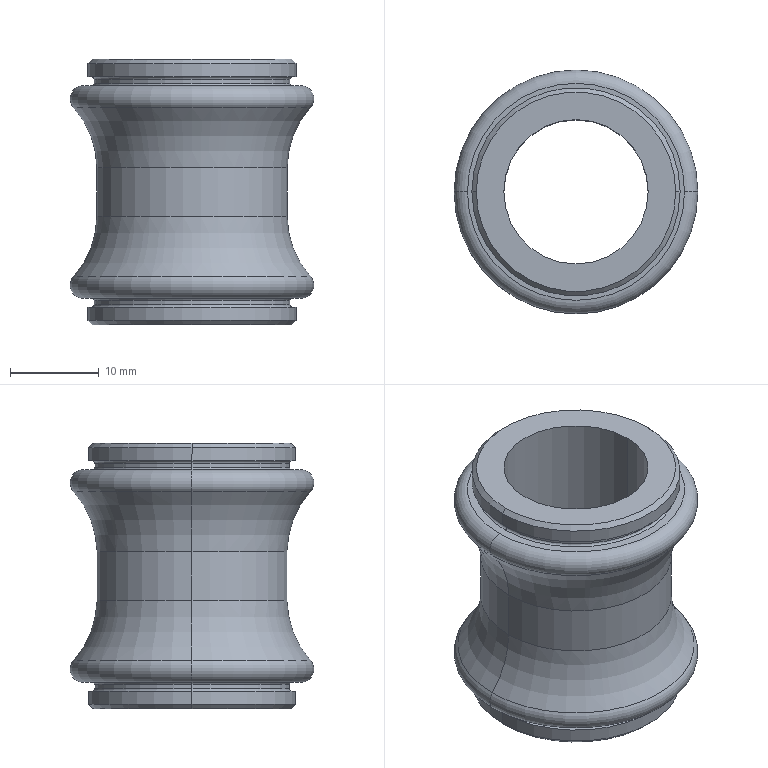Part | SolidWorks | features RefAxis 3, 3DProfileFeature 1, Revolution 1 | 1 solid | 38 faces | box 27.5 x 27.5 x 30 mm | volume 6795 mm3 | torus 16 | cylinder 12 | plane 6 | cone 4 | commonest cylinder face diameters 22.1 x4 23.5 x4 16.3 x2 21.5 x2
STEP:
#1=CARTESIAN_POINT('',(-8.15,0.,0.));
#2=VERTEX_POINT('',#1);
#3=CARTESIAN_POINT('',(8.15,0.,0.));
#4=VERTEX_POINT('',#3);
#5=CARTESIAN_POINT('',(0.,0.,0.));
#6=DIRECTION('',(0.,0.,1.));
#7=DIRECTION('',(1.,0.,0.));
#8=AXIS2_PLACEMENT_3D('',#5,#6,#7);
#9=CIRCLE('',#8,8.15);
#10=EDGE_CURVE('',#2,#4,#9,.T.);
#11=ORIENTED_EDGE('',*,*,#10,.F.);
#12=CARTESIAN_POINT('',(-8.15,0.,30.));
#13=VERTEX_POINT('',#12);
#14=CARTESIAN_POINT('',(-8.15,0.,0.));
#15=DIRECTION('',(0.,0.,1.));
#16=VECTOR('',#15,1000.);
#17=LINE('',#14,#16);
#18=EDGE_CURVE('',#2,#13,#17,.T.);
#19=ORIENTED_EDGE('',*,*,#18,.T.);
#20=CARTESIAN_POINT('',(8.15,0.,30.));
#21=VERTEX_POINT('',#20);
#22=CARTESIAN_POINT('',(0.,0.,30.));
#23=DIRECTION('',(0.,0.,1.));
#24=DIRECTION('',(1.,0.,0.));
#25=AXIS2_PLACEMENT_3D('',#22,#23,#24);
#26=CIRCLE('',#25,8.15);
#27=EDGE_CURVE('',#13,#21,#26,.T.);
#28=ORIENTED_EDGE('',*,*,#27,.T.);
#29=CARTESIAN_POINT('',(8.15,0.,0.));
#30=DIRECTION('',(0.,0.,1.));
#31=VECTOR('',#30,1000.);
#32=LINE('',#29,#31);
#33=EDGE_CURVE('',#4,#21,#32,.T.);
#34=ORIENTED_EDGE('',*,*,#33,.F.);
#35=EDGE_LOOP('',(#11,#19,#28,#34));
#36=FACE_OUTER_BOUND('',#35,.T.);
#37=CARTESIAN_POINT('',(0.,0.,0.));
#38=DIRECTION('',(0.,0.,1.));
#39=DIRECTION('',(1.,0.,0.));
#40=AXIS2_PLACEMENT_3D('',#37,#38,#39);
#41=CYLINDRICAL_SURFACE('',#40,8.15);
#42=ADVANCED_FACE('',(#36),#41,.F.);
#43=CARTESIAN_POINT('',(11.25,0.,0.));
#44=VERTEX_POINT('',#43);
#45=CARTESIAN_POINT('',(-11.25,0.,0.));
#46=VERTEX_POINT('',#45);
#47=CARTESIAN_POINT('',(0.,0.,0.));
#48=DIRECTION('',(0.,0.,1.));
#49=DIRECTION('',(1.,0.,0.));
#50=AXIS2_PLACEMENT_3D('',#47,#48,#49);
#51=CIRCLE('',#50,11.25);
#52=EDGE_CURVE('',#44,#46,#51,.T.);
#53=ORIENTED_EDGE('',*,*,#52,.T.);
#54=CARTESIAN_POINT('',(-11.75,0.,0.5));
#55=VERTEX_POINT('',#54);
#56=CARTESIAN_POINT('',(-11.25,0.,0.));
#57=DIRECTION('',(-0.7071,0.,0.7071));
#58=VECTOR('',#57,1000.);
#59=LINE('',#56,#58);
#60=EDGE_CURVE('',#46,#55,#59,.T.);
#61=ORIENTED_EDGE('',*,*,#60,.T.);
#62=CARTESIAN_POINT('',(11.75,0.,0.5));
#63=VERTEX_POINT('',#62);
#64=CARTESIAN_POINT('',(0.,0.,0.5));
#65=DIRECTION('',(0.,0.,1.));
#66=DIRECTION('',(1.,0.,0.));
#67=AXIS2_PLACEMENT_3D('',#64,#65,#66);
#68=CIRCLE('',#67,11.75);
#69=EDGE_CURVE('',#63,#55,#68,.T.);
#70=ORIENTED_EDGE('',*,*,#69,.F.);
#71=CARTESIAN_POINT('',(11.25,0.,0.));
#72=DIRECTION('',(0.7071,0.,0.7071));
#73=VECTOR('',#72,1000.);
#74=LINE('',#71,#73);
#75=EDGE_CURVE('',#44,#63,#74,.T.);
#76=ORIENTED_EDGE('',*,*,#75,.F.);
#77=EDGE_LOOP('',(#53,#61,#70,#76));
#78=FACE_OUTER_BOUND('',#77,.T.);
#79=CARTESIAN_POINT('',(0.,0.,0.));
#80=DIRECTION('',(0.,0.,1.));
#81=DIRECTION('',(1.,0.,0.));
#82=AXIS2_PLACEMENT_3D('',#79,#80,#81);
#83=CONICAL_SURFACE('',#82,11.25,0.7854);
#84=ADVANCED_FACE('',(#78),#83,.T.);
#85=ORIENTED_EDGE('',*,*,#69,.T.);
#86=CARTESIAN_POINT('',(-11.75,0.,2.));
#87=VERTEX_POINT('',#86);
#88=CARTESIAN_POINT('',(-11.75,0.,0.));
#89=DIRECTION('',(0.,0.,1.));
#90=VECTOR('',#89,1000.);
#91=LINE('',#88,#90);
#92=EDGE_CURVE('',#55,#87,#91,.T.);
#93=ORIENTED_EDGE('',*,*,#92,.T.);
#94=CARTESIAN_POINT('',(11.75,0.,2.));
#95=VERTEX_POINT('',#94);
#96=CARTESIAN_POINT('',(0.,0.,2.));
#97=DIRECTION('',(0.,0.,1.));
#98=DIRECTION('',(1.,0.,0.));
#99=AXIS2_PLACEMENT_3D('',#96,#97,#98);
#100=CIRCLE('',#99,11.75);
#101=EDGE_CURVE('',#95,#87,#100,.T.);
#102=ORIENTED_EDGE('',*,*,#101,.F.);
#103=CARTESIAN_POINT('',(11.75,0.,0.));
#104=DIRECTION('',(0.,0.,1.));
#105=VECTOR('',#104,1000.);
#106=LINE('',#103,#105);
#107=EDGE_CURVE('',#63,#95,#106,.T.);
#108=ORIENTED_EDGE('',*,*,#107,.F.);
#109=EDGE_LOOP('',(#85,#93,#102,#108));
#110=FACE_OUTER_BOUND('',#109,.T.);
#111=CARTESIAN_POINT('',(0.,0.,0.));
#112=DIRECTION('',(0.,0.,1.));
#113=DIRECTION('',(1.,0.,0.));
#114=AXIS2_PLACEMENT_3D('',#111,#112,#113);
#115=CYLINDRICAL_SURFACE('',#114,11.75);
#116=ADVANCED_FACE('',(#110),#115,.T.);
#117=CARTESIAN_POINT('',(-11.05,0.,2.25));
#118=VERTEX_POINT('',#117);
#119=CARTESIAN_POINT('',(11.05,0.,2.25));
#120=VERTEX_POINT('',#119);
#121=CARTESIAN_POINT('',(0.,0.,2.25));
#122=DIRECTION('',(0.,0.,1.));
#123=DIRECTION('',(1.,0.,0.));
#124=AXIS2_PLACEMENT_3D('',#121,#122,#123);
#125=CIRCLE('',#124,11.05);
#126=EDGE_CURVE('',#118,#120,#125,.T.);
#127=ORIENTED_EDGE('',*,*,#126,.F.);
#128=CARTESIAN_POINT('',(-11.3,0.,2.));
#129=VERTEX_POINT('',#128);
#130=CARTESIAN_POINT('',(-11.3,0.,2.25));
#131=DIRECTION('',(0.,1.,0.));
#132=DIRECTION('',(-1.,0.,0.));
#133=AXIS2_PLACEMENT_3D('',#130,#131,#132);
#134=CIRCLE('',#133,0.25);
#135=EDGE_CURVE('',#118,#129,#134,.T.);
#136=ORIENTED_EDGE('',*,*,#135,.T.);
#137=CARTESIAN_POINT('',(11.3,0.,2.));
#138=VERTEX_POINT('',#137);
#139=CARTESIAN_POINT('',(0.,0.,2.));
#140=DIRECTION('',(0.,0.,1.));
#141=DIRECTION('',(1.,0.,0.));
#142=AXIS2_PLACEMENT_3D('',#139,#140,#141);
#143=CIRCLE('',#142,11.3);
#144=EDGE_CURVE('',#129,#138,#143,.T.);
#145=ORIENTED_EDGE('',*,*,#144,.T.);
#146=CARTESIAN_POINT('',(11.3,0.,2.25));
#147=DIRECTION('',(0.,-1.,0.));
#148=DIRECTION('',(0.,0.,-1.));
#149=AXIS2_PLACEMENT_3D('',#146,#147,#148);
#150=CIRCLE('',#149,0.25);
#151=EDGE_CURVE('',#120,#138,#150,.T.);
#152=ORIENTED_EDGE('',*,*,#151,.F.);
#153=EDGE_LOOP('',(#127,#136,#145,#152));
#154=FACE_OUTER_BOUND('',#153,.T.);
#155=CARTESIAN_POINT('',(0.,0.,2.25));
#156=DIRECTION('',(0.,0.,1.));
#157=DIRECTION('',(1.,0.,0.));
#158=AXIS2_PLACEMENT_3D('',#155,#156,#157);
#159=TOROIDAL_SURFACE('',#158,11.3,0.25);
#160=ADVANCED_FACE('',(#154),#159,.F.);
#161=CARTESIAN_POINT('',(0.,0.,2.25));
#162=DIRECTION('',(0.,0.,1.));
#163=DIRECTION('',(1.,0.,0.));
#164=AXIS2_PLACEMENT_3D('',#161,#162,#163);
#165=CIRCLE('',#164,11.05);
#166=EDGE_CURVE('',#120,#118,#165,.T.);
#167=ORIENTED_EDGE('',*,*,#166,.T.);
#168=CARTESIAN_POINT('',(-11.05,0.,2.75));
#169=VERTEX_POINT('',#168);
#170=CARTESIAN_POINT('',(-11.05,0.,0.));
#171=DIRECTION('',(0.,0.,1.));
#172=VECTOR('',#171,1000.);
#173=LINE('',#170,#172);
#174=EDGE_CURVE('',#118,#169,#173,.T.);
#175=ORIENTED_EDGE('',*,*,#174,.T.);
#176=CARTESIAN_POINT('',(11.05,0.,2.75));
#177=VERTEX_POINT('',#176);
#178=CARTESIAN_POINT('',(0.,0.,2.75));
#179=DIRECTION('',(0.,0.,1.));
#180=DIRECTION('',(1.,0.,0.));
#181=AXIS2_PLACEMENT_3D('',#178,#179,#180);
#182=CIRCLE('',#181,11.05);
#183=EDGE_CURVE('',#177,#169,#182,.T.);
#184=ORIENTED_EDGE('',*,*,#183,.F.);
#185=CARTESIAN_POINT('',(11.05,0.,0.));
#186=DIRECTION('',(0.,0.,1.));
#187=VECTOR('',#186,1000.);
#188=LINE('',#185,#187);
#189=EDGE_CURVE('',#120,#177,#188,.T.);
#190=ORIENTED_EDGE('',*,*,#189,.F.);
#191=EDGE_LOOP('',(#167,#175,#184,#190));
#192=FACE_OUTER_BOUND('',#191,.T.);
#193=CARTESIAN_POINT('',(0.,0.,0.));
#194=DIRECTION('',(0.,0.,1.));
#195=DIRECTION('',(1.,0.,0.));
#196=AXIS2_PLACEMENT_3D('',#193,#194,#195);
#197=CYLINDRICAL_SURFACE('',#196,11.05);
#198=ADVANCED_FACE('',(#192),#197,.T.);
#199=CARTESIAN_POINT('',(-11.3,0.,3.));
#200=VERTEX_POINT('',#199);
#201=CARTESIAN_POINT('',(11.3,0.,3.));
#202=VERTEX_POINT('',#201);
#203=CARTESIAN_POINT('',(0.,0.,3.));
#204=DIRECTION('',(0.,0.,1.));
#205=DIRECTION('',(1.,0.,0.));
#206=AXIS2_PLACEMENT_3D('',#203,#204,#205);
#207=CIRCLE('',#206,11.3);
#208=EDGE_CURVE('',#200,#202,#207,.T.);
#209=ORIENTED_EDGE('',*,*,#208,.F.);
#210=CARTESIAN_POINT('',(-11.3,0.,2.75));
#211=DIRECTION('',(0.,1.,0.));
#212=DIRECTION('',(-1.,0.,0.));
#213=AXIS2_PLACEMENT_3D('',#210,#211,#212);
#214=CIRCLE('',#213,0.25);
#215=EDGE_CURVE('',#200,#169,#214,.T.);
#216=ORIENTED_EDGE('',*,*,#215,.T.);
#217=CARTESIAN_POINT('',(0.,0.,2.75));
#218=DIRECTION('',(0.,0.,1.));
#219=DIRECTION('',(1.,0.,0.));
#220=AXIS2_PLACEMENT_3D('',#217,#218,#219);
#221=CIRCLE('',#220,11.05);
#222=EDGE_CURVE('',#169,#177,#221,.T.);
#223=ORIENTED_EDGE('',*,*,#222,.T.);
#224=CARTESIAN_POINT('',(11.3,0.,2.75));
#225=DIRECTION('',(0.,-1.,0.));
#226=DIRECTION('',(0.,0.,-1.));
#227=AXIS2_PLACEMENT_3D('',#224,#225,#226);
#228=CIRCLE('',#227,0.25);
#229=EDGE_CURVE('',#202,#177,#228,.T.);
#230=ORIENTED_EDGE('',*,*,#229,.F.);
#231=EDGE_LOOP('',(#209,#216,#223,#230));
#232=FACE_OUTER_BOUND('',#231,.T.);
#233=CARTESIAN_POINT('',(0.,0.,2.75));
#234=DIRECTION('',(0.,0.,1.));
#235=DIRECTION('',(1.,0.,0.));
#236=AXIS2_PLACEMENT_3D('',#233,#234,#235);
#237=TOROIDAL_SURFACE('',#236,11.3,0.25);
#238=ADVANCED_FACE('',(#232),#237,.F.);
#239=CARTESIAN_POINT('',(12.25,0.,3.));
#240=VERTEX_POINT('',#239);
#241=CARTESIAN_POINT('',(-12.25,0.,3.));
#242=VERTEX_POINT('',#241);
#243=CARTESIAN_POINT('',(0.,0.,3.));
#244=DIRECTION('',(0.,0.,1.));
#245=DIRECTION('',(1.,0.,0.));
#246=AXIS2_PLACEMENT_3D('',#243,#244,#245);
#247=CIRCLE('',#246,12.25);
#248=EDGE_CURVE('',#240,#242,#247,.T.);
#249=ORIENTED_EDGE('',*,*,#248,.T.);
#250=CARTESIAN_POINT('',(-13.359,0.,5.51));
#251=VERTEX_POINT('',#250);
#252=CARTESIAN_POINT('',(-12.25,0.,4.5));
#253=DIRECTION('',(0.,1.,0.));
#254=DIRECTION('',(-1.,0.,0.));
#255=AXIS2_PLACEMENT_3D('',#252,#253,#254);
#256=CIRCLE('',#255,1.5);
#257=EDGE_CURVE('',#242,#251,#256,.T.);
#258=ORIENTED_EDGE('',*,*,#257,.T.);
#259=CARTESIAN_POINT('',(13.359,0.,5.51));
#260=VERTEX_POINT('',#259);
#261=CARTESIAN_POINT('',(0.,0.,5.51));
#262=DIRECTION('',(0.,0.,1.));
#263=DIRECTION('',(1.,0.,0.));
#264=AXIS2_PLACEMENT_3D('',#261,#262,#263);
#265=CIRCLE('',#264,13.359);
#266=EDGE_CURVE('',#260,#251,#265,.T.);
#267=ORIENTED_EDGE('',*,*,#266,.F.);
#268=CARTESIAN_POINT('',(12.25,0.,4.5));
#269=DIRECTION('',(0.,-1.,0.));
#270=DIRECTION('',(0.,0.,-1.));
#271=AXIS2_PLACEMENT_3D('',#268,#269,#270);
#272=CIRCLE('',#271,1.5);
#273=EDGE_CURVE('',#240,#260,#272,.T.);
#274=ORIENTED_EDGE('',*,*,#273,.F.);
#275=EDGE_LOOP('',(#249,#258,#267,#274));
#276=FACE_OUTER_BOUND('',#275,.T.);
#277=CARTESIAN_POINT('',(0.,0.,4.5));
#278=DIRECTION('',(0.,0.,1.));
#279=DIRECTION('',(1.,0.,0.));
#280=AXIS2_PLACEMENT_3D('',#277,#278,#279);
#281=TOROIDAL_SURFACE('',#280,12.25,1.5);
#282=ADVANCED_FACE('',(#276),#281,.T.);
#283=CARTESIAN_POINT('',(-10.75,0.,12.246));
#284=VERTEX_POINT('',#283);
#285=CARTESIAN_POINT('',(10.75,0.,12.246));
#286=VERTEX_POINT('',#285);
#287=CARTESIAN_POINT('',(0.,0.,12.246));
#288=DIRECTION('',(0.,0.,1.));
#289=DIRECTION('',(1.,0.,0.));
#290=AXIS2_PLACEMENT_3D('',#287,#288,#289);
#291=CIRCLE('',#290,10.75);
#292=EDGE_CURVE('',#284,#286,#291,.T.);
#293=ORIENTED_EDGE('',*,*,#292,.F.);
#294=CARTESIAN_POINT('',(-20.75,0.,12.246));
#295=DIRECTION('',(0.,1.,0.));
#296=DIRECTION('',(-1.,0.,0.));
#297=AXIS2_PLACEMENT_3D('',#294,#295,#296);
#298=CIRCLE('',#297,10.);
#299=EDGE_CURVE('',#284,#251,#298,.T.);
#300=ORIENTED_EDGE('',*,*,#299,.T.);
#301=CARTESIAN_POINT('',(0.,0.,5.51));
#302=DIRECTION('',(0.,0.,1.));
#303=DIRECTION('',(1.,0.,0.));
#304=AXIS2_PLACEMENT_3D('',#301,#302,#303);
#305=CIRCLE('',#304,13.359);
#306=EDGE_CURVE('',#251,#260,#305,.T.);
#307=ORIENTED_EDGE('',*,*,#306,.T.);
#308=CARTESIAN_POINT('',(20.75,0.,12.246));
#309=DIRECTION('',(0.,-1.,0.));
#310=DIRECTION('',(0.,0.,-1.));
#311=AXIS2_PLACEMENT_3D('',#308,#309,#310);
#312=CIRCLE('',#311,10.);
#313=EDGE_CURVE('',#286,#260,#312,.T.);
#314=ORIENTED_EDGE('',*,*,#313,.F.);
#315=EDGE_LOOP('',(#293,#300,#307,#314));
#316=FACE_OUTER_BOUND('',#315,.T.);
#317=CARTESIAN_POINT('',(0.,0.,12.246));
#318=DIRECTION('',(0.,0.,1.));
#319=DIRECTION('',(1.,0.,0.));
#320=AXIS2_PLACEMENT_3D('',#317,#318,#319);
#321=TOROIDAL_SURFACE('',#320,20.75,10.);
#322=ADVANCED_FACE('',(#316),#321,.F.);
#323=CARTESIAN_POINT('',(0.,0.,12.246));
#324=DIRECTION('',(0.,0.,1.));
#325=DIRECTION('',(1.,0.,0.));
#326=AXIS2_PLACEMENT_3D('',#323,#324,#325);
#327=CIRCLE('',#326,10.75);
#328=EDGE_CURVE('',#286,#284,#327,.T.);
#329=ORIENTED_EDGE('',*,*,#328,.T.);
#330=CARTESIAN_POINT('',(-10.75,0.,17.754));
#331=VERTEX_POINT('',#330);
#332=CARTESIAN_POINT('',(-10.75,0.,0.));
#333=DIRECTION('',(0.,0.,1.));
#334=VECTOR('',#333,1000.);
#335=LINE('',#332,#334);
#336=EDGE_CURVE('',#284,#331,#335,.T.);
#337=ORIENTED_EDGE('',*,*,#336,.T.);
#338=CARTESIAN_POINT('',(10.75,0.,17.754));
#339=VERTEX_POINT('',#338);
#340=CARTESIAN_POINT('',(0.,0.,17.754));
#341=DIRECTION('',(0.,0.,1.));
#342=DIRECTION('',(1.,0.,0.));
#343=AXIS2_PLACEMENT_3D('',#340,#341,#342);
#344=CIRCLE('',#343,10.75);
#345=EDGE_CURVE('',#339,#331,#344,.T.);
#346=ORIENTED_EDGE('',*,*,#345,.F.);
#347=CARTESIAN_POINT('',(10.75,0.,0.));
#348=DIRECTION('',(0.,0.,1.));
#349=VECTOR('',#348,1000.);
#350=LINE('',#347,#349);
#351=EDGE_CURVE('',#286,#339,#350,.T.);
#352=ORIENTED_EDGE('',*,*,#351,.F.);
#353=EDGE_LOOP('',(#329,#337,#346,#352));
#354=FACE_OUTER_BOUND('',#353,.T.);
#355=CARTESIAN_POINT('',(0.,0.,0.));
#356=DIRECTION('',(0.,0.,1.));
#357=DIRECTION('',(1.,0.,0.));
#358=AXIS2_PLACEMENT_3D('',#355,#356,#357);
#359=CYLINDRICAL_SURFACE('',#358,10.75);
#360=ADVANCED_FACE('',(#354),#359,.T.);
#361=CARTESIAN_POINT('',(-13.359,0.,24.49));
#362=VERTEX_POINT('',#361);
#363=CARTESIAN_POINT('',(13.359,0.,24.49));
#364=VERTEX_POINT('',#363);
#365=CARTESIAN_POINT('',(0.,0.,24.49));
#366=DIRECTION('',(0.,0.,1.));
#367=DIRECTION('',(1.,0.,0.));
#368=AXIS2_PLACEMENT_3D('',#365,#366,#367);
#369=CIRCLE('',#368,13.359);
#370=EDGE_CURVE('',#362,#364,#369,.T.);
#371=ORIENTED_EDGE('',*,*,#370,.F.);
#372=CARTESIAN_POINT('',(-20.75,0.,17.754));
#373=DIRECTION('',(0.,1.,0.));
#374=DIRECTION('',(-1.,0.,0.));
#375=AXIS2_PLACEMENT_3D('',#372,#373,#374);
#376=CIRCLE('',#375,10.);
#377=EDGE_CURVE('',#362,#331,#376,.T.);
#378=ORIENTED_EDGE('',*,*,#377,.T.);
#379=CARTESIAN_POINT('',(0.,0.,17.754));
#380=DIRECTION('',(0.,0.,1.));
#381=DIRECTION('',(1.,0.,0.));
#382=AXIS2_PLACEMENT_3D('',#379,#380,#381);
#383=CIRCLE('',#382,10.75);
#384=EDGE_CURVE('',#331,#339,#383,.T.);
#385=ORIENTED_EDGE('',*,*,#384,.T.);
#386=CARTESIAN_POINT('',(20.75,0.,17.754));
#387=DIRECTION('',(0.,-1.,0.));
#388=DIRECTION('',(0.,0.,-1.));
#389=AXIS2_PLACEMENT_3D('',#386,#387,#388);
#390=CIRCLE('',#389,10.);
#391=EDGE_CURVE('',#364,#339,#390,.T.);
#392=ORIENTED_EDGE('',*,*,#391,.F.);
#393=EDGE_LOOP('',(#371,#378,#385,#392));
#394=FACE_OUTER_BOUND('',#393,.T.);
#395=CARTESIAN_POINT('',(0.,0.,17.754));
#396=DIRECTION('',(0.,0.,1.));
#397=DIRECTION('',(1.,0.,0.));
#398=AXIS2_PLACEMENT_3D('',#395,#396,#397);
#399=TOROIDAL_SURFACE('',#398,20.75,10.);
#400=ADVANCED_FACE('',(#394),#399,.F.);
#401=CARTESIAN_POINT('',(0.,0.,24.49));
#402=DIRECTION('',(0.,0.,1.));
#403=DIRECTION('',(1.,0.,0.));
#404=AXIS2_PLACEMENT_3D('',#401,#402,#403);
#405=CIRCLE('',#404,13.359);
#406=EDGE_CURVE('',#364,#362,#405,.T.);
#407=ORIENTED_EDGE('',*,*,#406,.T.);
#408=CARTESIAN_POINT('',(-12.25,0.,27.));
#409=VERTEX_POINT('',#408);
#410=CARTESIAN_POINT('',(-12.25,0.,25.5));
#411=DIRECTION('',(0.,1.,0.));
#412=DIRECTION('',(-1.,0.,0.));
#413=AXIS2_PLACEMENT_3D('',#410,#411,#412);
#414=CIRCLE('',#413,1.5);
#415=EDGE_CURVE('',#362,#409,#414,.T.);
#416=ORIENTED_EDGE('',*,*,#415,.T.);
#417=CARTESIAN_POINT('',(12.25,0.,27.));
#418=VERTEX_POINT('',#417);
#419=CARTESIAN_POINT('',(0.,0.,27.));
#420=DIRECTION('',(0.,0.,1.));
#421=DIRECTION('',(1.,0.,0.));
#422=AXIS2_PLACEMENT_3D('',#419,#420,#421);
#423=CIRCLE('',#422,12.25);
#424=EDGE_CURVE('',#418,#409,#423,.T.);
#425=ORIENTED_EDGE('',*,*,#424,.F.);
#426=CARTESIAN_POINT('',(12.25,0.,25.5));
#427=DIRECTION('',(0.,-1.,0.));
#428=DIRECTION('',(0.,0.,-1.));
#429=AXIS2_PLACEMENT_3D('',#426,#427,#428);
#430=CIRCLE('',#429,1.5);
#431=EDGE_CURVE('',#364,#418,#430,.T.);
#432=ORIENTED_EDGE('',*,*,#431,.F.);
#433=EDGE_LOOP('',(#407,#416,#425,#432));
#434=FACE_OUTER_BOUND('',#433,.T.);
#435=CARTESIAN_POINT('',(0.,0.,25.5));
#436=DIRECTION('',(0.,0.,1.));
#437=DIRECTION('',(1.,0.,0.));
#438=AXIS2_PLACEMENT_3D('',#435,#436,#437);
#439=TOROIDAL_SURFACE('',#438,12.25,1.5);
#440=ADVANCED_FACE('',(#434),#439,.T.);
#441=CARTESIAN_POINT('',(-11.05,0.,27.25));
#442=VERTEX_POINT('',#441);
#443=CARTESIAN_POINT('',(11.05,0.,27.25));
#444=VERTEX_POINT('',#443);
#445=CARTESIAN_POINT('',(0.,0.,27.25));
#446=DIRECTION('',(0.,0.,1.));
#447=DIRECTION('',(1.,0.,0.));
#448=AXIS2_PLACEMENT_3D('',#445,#446,#447);
#449=CIRCLE('',#448,11.05);
#450=EDGE_CURVE('',#442,#444,#449,.T.);
#451=ORIENTED_EDGE('',*,*,#450,.F.);
#452=CARTESIAN_POINT('',(-11.3,0.,27.));
#453=VERTEX_POINT('',#452);
#454=CARTESIAN_POINT('',(-11.3,0.,27.25));
#455=DIRECTION('',(0.,1.,0.));
#456=DIRECTION('',(-1.,0.,0.));
#457=AXIS2_PLACEMENT_3D('',#454,#455,#456);
#458=CIRCLE('',#457,0.25);
#459=EDGE_CURVE('',#442,#453,#458,.T.);
#460=ORIENTED_EDGE('',*,*,#459,.T.);
#461=CARTESIAN_POINT('',(11.3,0.,27.));
#462=VERTEX_POINT('',#461);
#463=CARTESIAN_POINT('',(0.,0.,27.));
#464=DIRECTION('',(0.,0.,1.));
#465=DIRECTION('',(1.,0.,0.));
#466=AXIS2_PLACEMENT_3D('',#463,#464,#465);
#467=CIRCLE('',#466,11.3);
#468=EDGE_CURVE('',#453,#462,#467,.T.);
#469=ORIENTED_EDGE('',*,*,#468,.T.);
#470=CARTESIAN_POINT('',(11.3,0.,27.25));
#471=DIRECTION('',(0.,-1.,0.));
#472=DIRECTION('',(0.,0.,-1.));
#473=AXIS2_PLACEMENT_3D('',#470,#471,#472);
#474=CIRCLE('',#473,0.25);
#475=EDGE_CURVE('',#444,#462,#474,.T.);
#476=ORIENTED_EDGE('',*,*,#475,.F.);
#477=EDGE_LOOP('',(#451,#460,#469,#476));
#478=FACE_OUTER_BOUND('',#477,.T.);
#479=CARTESIAN_POINT('',(0.,0.,27.25));
#480=DIRECTION('',(0.,0.,1.));
#481=DIRECTION('',(1.,0.,0.));
#482=AXIS2_PLACEMENT_3D('',#479,#480,#481);
#483=TOROIDAL_SURFACE('',#482,11.3,0.25);
#484=ADVANCED_FACE('',(#478),#483,.F.);
#485=CARTESIAN_POINT('',(0.,0.,27.25));
#486=DIRECTION('',(0.,0.,1.));
#487=DIRECTION('',(1.,0.,0.));
#488=AXIS2_PLACEMENT_3D('',#485,#486,#487);
#489=CIRCLE('',#488,11.05);
#490=EDGE_CURVE('',#444,#442,#489,.T.);
#491=ORIENTED_EDGE('',*,*,#490,.T.);
#492=CARTESIAN_POINT('',(-11.05,0.,27.75));
#493=VERTEX_POINT('',#492);
#494=CARTESIAN_POINT('',(-11.05,0.,0.));
#495=DIRECTION('',(0.,0.,1.));
#496=VECTOR('',#495,1000.);
#497=LINE('',#494,#496);
#498=EDGE_CURVE('',#442,#493,#497,.T.);
#499=ORIENTED_EDGE('',*,*,#498,.T.);
#500=CARTESIAN_POINT('',(11.05,0.,27.75));
#501=VERTEX_POINT('',#500);
#502=CARTESIAN_POINT('',(0.,0.,27.75));
#503=DIRECTION('',(0.,0.,1.));
#504=DIRECTION('',(1.,0.,0.));
#505=AXIS2_PLACEMENT_3D('',#502,#503,#504);
#506=CIRCLE('',#505,11.05);
#507=EDGE_CURVE('',#501,#493,#506,.T.);
#508=ORIENTED_EDGE('',*,*,#507,.F.);
#509=CARTESIAN_POINT('',(11.05,0.,0.));
#510=DIRECTION('',(0.,0.,1.));
#511=VECTOR('',#510,1000.);
#512=LINE('',#509,#511);
#513=EDGE_CURVE('',#444,#501,#512,.T.);
#514=ORIENTED_EDGE('',*,*,#513,.F.);
#515=EDGE_LOOP('',(#491,#499,#508,#514));
#516=FACE_OUTER_BOUND('',#515,.T.);
#517=CARTESIAN_POINT('',(0.,0.,0.));
#518=DIRECTION('',(0.,0.,1.));
#519=DIRECTION('',(1.,0.,0.));
#520=AXIS2_PLACEMENT_3D('',#517,#518,#519);
#521=CYLINDRICAL_SURFACE('',#520,11.05);
#522=ADVANCED_FACE('',(#516),#521,.T.);
#523=CARTESIAN_POINT('',(-11.3,0.,28.));
#524=VERTEX_POINT('',#523);
#525=CARTESIAN_POINT('',(11.3,0.,28.));
#526=VERTEX_POINT('',#525);
#527=CARTESIAN_POINT('',(0.,0.,28.));
#528=DIRECTION('',(0.,0.,1.));
#529=DIRECTION('',(1.,0.,0.));
#530=AXIS2_PLACEMENT_3D('',#527,#528,#529);
#531=CIRCLE('',#530,11.3);
#532=EDGE_CURVE('',#524,#526,#531,.T.);
#533=ORIENTED_EDGE('',*,*,#532,.F.);
#534=CARTESIAN_POINT('',(-11.3,0.,27.75));
#535=DIRECTION('',(0.,1.,0.));
#536=DIRECTION('',(-1.,0.,0.));
#537=AXIS2_PLACEMENT_3D('',#534,#535,#536);
#538=CIRCLE('',#537,0.25);
#539=EDGE_CURVE('',#524,#493,#538,.T.);
#540=ORIENTED_EDGE('',*,*,#539,.T.);
#541=CARTESIAN_POINT('',(0.,0.,27.75));
#542=DIRECTION('',(0.,0.,1.));
#543=DIRECTION('',(1.,0.,0.));
#544=AXIS2_PLACEMENT_3D('',#541,#542,#543);
#545=CIRCLE('',#544,11.05);
#546=EDGE_CURVE('',#493,#501,#545,.T.);
#547=ORIENTED_EDGE('',*,*,#546,.T.);
#548=CARTESIAN_POINT('',(11.3,0.,27.75));
#549=DIRECTION('',(0.,-1.,0.));
#550=DIRECTION('',(0.,0.,-1.));
#551=AXIS2_PLACEMENT_3D('',#548,#549,#550);
#552=CIRCLE('',#551,0.25);
#553=EDGE_CURVE('',#526,#501,#552,.T.);
#554=ORIENTED_EDGE('',*,*,#553,.F.);
#555=EDGE_LOOP('',(#533,#540,#547,#554));
#556=FACE_OUTER_BOUND('',#555,.T.);
#557=CARTESIAN_POINT('',(0.,0.,27.75));
#558=DIRECTION('',(0.,0.,1.));
#559=DIRECTION('',(1.,0.,0.));
#560=AXIS2_PLACEMENT_3D('',#557,#558,#559);
#561=TOROIDAL_SURFACE('',#560,11.3,0.25);
#562=ADVANCED_FACE('',(#556),#561,.F.);
#563=CARTESIAN_POINT('',(11.75,0.,28.));
#564=VERTEX_POINT('',#563);
#565=CARTESIAN_POINT('',(-11.75,0.,28.));
#566=VERTEX_POINT('',#565);
#567=CARTESIAN_POINT('',(0.,0.,28.));
#568=DIRECTION('',(0.,0.,1.));
#569=DIRECTION('',(1.,0.,0.));
#570=AXIS2_PLACEMENT_3D('',#567,#568,#569);
#571=CIRCLE('',#570,11.75);
#572=EDGE_CURVE('',#564,#566,#571,.T.);
#573=ORIENTED_EDGE('',*,*,#572,.T.);
#574=CARTESIAN_POINT('',(-11.75,0.,29.5));
#575=VERTEX_POINT('',#574);
#576=CARTESIAN_POINT('',(-11.75,0.,0.));
#577=DIRECTION('',(0.,0.,1.));
#578=VECTOR('',#577,1000.);
#579=LINE('',#576,#578);
#580=EDGE_CURVE('',#566,#575,#579,.T.);
#581=ORIENTED_EDGE('',*,*,#580,.T.);
#582=CARTESIAN_POINT('',(11.75,0.,29.5));
#583=VERTEX_POINT('',#582);
#584=CARTESIAN_POINT('',(0.,0.,29.5));
#585=DIRECTION('',(0.,0.,1.));
#586=DIRECTION('',(1.,0.,0.));
#587=AXIS2_PLACEMENT_3D('',#584,#585,#586);
#588=CIRCLE('',#587,11.75);
#589=EDGE_CURVE('',#583,#575,#588,.T.);
#590=ORIENTED_EDGE('',*,*,#589,.F.);
#591=CARTESIAN_POINT('',(11.75,0.,0.));
#592=DIRECTION('',(0.,0.,1.));
#593=VECTOR('',#592,1000.);
#594=LINE('',#591,#593);
#595=EDGE_CURVE('',#564,#583,#594,.T.);
#596=ORIENTED_EDGE('',*,*,#595,.F.);
#597=EDGE_LOOP('',(#573,#581,#590,#596));
#598=FACE_OUTER_BOUND('',#597,.T.);
#599=CARTESIAN_POINT('',(0.,0.,0.));
#600=DIRECTION('',(0.,0.,1.));
#601=DIRECTION('',(1.,0.,0.));
#602=AXIS2_PLACEMENT_3D('',#599,#600,#601);
#603=CYLINDRICAL_SURFACE('',#602,11.75);
#604=ADVANCED_FACE('',(#598),#603,.T.);
#605=CARTESIAN_POINT('',(11.25,0.,30.));
#606=VERTEX_POINT('',#605);
#607=CARTESIAN_POINT('',(-11.25,0.,30.));
#608=VERTEX_POINT('',#607);
#609=CARTESIAN_POINT('',(0.,0.,30.));
#610=DIRECTION('',(0.,0.,1.));
#611=DIRECTION('',(1.,0.,0.));
#612=AXIS2_PLACEMENT_3D('',#609,#610,#611);
#613=CIRCLE('',#612,11.25);
#614=EDGE_CURVE('',#606,#608,#613,.T.);
#615=ORIENTED_EDGE('',*,*,#614,.F.);
#616=CARTESIAN_POINT('',(11.75,0.,29.5));
#617=DIRECTION('',(0.7071,0.,-0.7071));
#618=VECTOR('',#617,1000.);
#619=LINE('',#616,#618);
#620=EDGE_CURVE('',#606,#583,#619,.T.);
#621=ORIENTED_EDGE('',*,*,#620,.T.);
#622=ORIENTED_EDGE('',*,*,#589,.T.);
#623=CARTESIAN_POINT('',(-11.75,0.,29.5));
#624=DIRECTION('',(-0.7071,0.,-0.7071));
#625=VECTOR('',#624,1000.);
#626=LINE('',#623,#625);
#627=EDGE_CURVE('',#608,#575,#626,.T.);
#628=ORIENTED_EDGE('',*,*,#627,.F.);
#629=EDGE_LOOP('',(#615,#621,#622,#628));
#630=FACE_OUTER_BOUND('',#629,.T.);
#631=CARTESIAN_POINT('',(0.,0.,29.5));
#632=DIRECTION('',(0.,0.,-1.));
#633=DIRECTION('',(-1.,0.,0.));
#634=AXIS2_PLACEMENT_3D('',#631,#632,#633);
#635=CONICAL_SURFACE('',#634,11.75,0.7854);
#636=ADVANCED_FACE('',(#630),#635,.T.);
#637=ORIENTED_EDGE('',*,*,#620,.F.);
#638=CARTESIAN_POINT('',(0.,0.,30.));
#639=DIRECTION('',(0.,0.,1.));
#640=DIRECTION('',(1.,0.,0.));
#641=AXIS2_PLACEMENT_3D('',#638,#639,#640);
#642=CIRCLE('',#641,11.25);
#643=EDGE_CURVE('',#608,#606,#642,.T.);
#644=ORIENTED_EDGE('',*,*,#643,.F.);
#645=ORIENTED_EDGE('',*,*,#627,.T.);
#646=CARTESIAN_POINT('',(0.,0.,29.5));
#647=DIRECTION('',(0.,0.,1.));
#648=DIRECTION('',(1.,0.,0.));
#649=AXIS2_PLACEMENT_3D('',#646,#647,#648);
#650=CIRCLE('',#649,11.75);
#651=EDGE_CURVE('',#575,#583,#650,.T.);
#652=ORIENTED_EDGE('',*,*,#651,.T.);
#653=EDGE_LOOP('',(#637,#644,#645,#652));
#654=FACE_OUTER_BOUND('',#653,.T.);
#655=CARTESIAN_POINT('',(0.,0.,29.5));
#656=DIRECTION('',(0.,0.,-1.));
#657=DIRECTION('',(-1.,0.,0.));
#658=AXIS2_PLACEMENT_3D('',#655,#656,#657);
#659=CONICAL_SURFACE('',#658,11.75,0.7854);
#660=ADVANCED_FACE('',(#654),#659,.T.);
#661=ORIENTED_EDGE('',*,*,#580,.F.);
#662=CARTESIAN_POINT('',(0.,0.,28.));
#663=DIRECTION('',(0.,0.,1.));
#664=DIRECTION('',(1.,0.,0.));
#665=AXIS2_PLACEMENT_3D('',#662,#663,#664);
#666=CIRCLE('',#665,11.75);
#667=EDGE_CURVE('',#566,#564,#666,.T.);
#668=ORIENTED_EDGE('',*,*,#667,.T.);
#669=ORIENTED_EDGE('',*,*,#595,.T.);
#670=ORIENTED_EDGE('',*,*,#651,.F.);
#671=EDGE_LOOP('',(#661,#668,#669,#670));
#672=FACE_OUTER_BOUND('',#671,.T.);
#673=CARTESIAN_POINT('',(0.,0.,0.));
#674=DIRECTION('',(0.,0.,1.));
#675=DIRECTION('',(1.,0.,0.));
#676=AXIS2_PLACEMENT_3D('',#673,#674,#675);
#677=CYLINDRICAL_SURFACE('',#676,11.75);
#678=ADVANCED_FACE('',(#672),#677,.T.);
#679=ORIENTED_EDGE('',*,*,#572,.F.);
#680=ORIENTED_EDGE('',*,*,#667,.F.);
#681=EDGE_LOOP('',(#679,#680));
#682=FACE_OUTER_BOUND('',#681,.T.);
#683=CARTESIAN_POINT('',(0.,0.,28.));
#684=DIRECTION('',(0.,0.,1.));
#685=DIRECTION('',(1.,0.,0.));
#686=AXIS2_PLACEMENT_3D('',#683,#684,#685);
#687=CIRCLE('',#686,11.3);
#688=EDGE_CURVE('',#526,#524,#687,.T.);
#689=ORIENTED_EDGE('',*,*,#688,.T.);
#690=ORIENTED_EDGE('',*,*,#532,.T.);
#691=EDGE_LOOP('',(#689,#690));
#692=FACE_BOUND('',#691,.T.);
#693=CARTESIAN_POINT('',(0.,11.3,28.));
#694=DIRECTION('',(0.,0.,1.));
#695=DIRECTION('',(1.,0.,0.));
#696=AXIS2_PLACEMENT_3D('',#693,#694,#695);
#697=PLANE('',#696);
#698=ADVANCED_FACE('',(#682,#692),#697,.F.);
#699=ORIENTED_EDGE('',*,*,#539,.F.);
#700=ORIENTED_EDGE('',*,*,#688,.F.);
#701=ORIENTED_EDGE('',*,*,#553,.T.);
#702=ORIENTED_EDGE('',*,*,#507,.T.);
#703=EDGE_LOOP('',(#699,#700,#701,#702));
#704=FACE_OUTER_BOUND('',#703,.T.);
#705=CARTESIAN_POINT('',(0.,0.,27.75));
#706=DIRECTION('',(0.,0.,1.));
#707=DIRECTION('',(1.,0.,0.));
#708=AXIS2_PLACEMENT_3D('',#705,#706,#707);
#709=TOROIDAL_SURFACE('',#708,11.3,0.25);
#710=ADVANCED_FACE('',(#704),#709,.F.);
#711=ORIENTED_EDGE('',*,*,#498,.F.);
#712=ORIENTED_EDGE('',*,*,#450,.T.);
#713=ORIENTED_EDGE('',*,*,#513,.T.);
#714=ORIENTED_EDGE('',*,*,#546,.F.);
#715=EDGE_LOOP('',(#711,#712,#713,#714));
#716=FACE_OUTER_BOUND('',#715,.T.);
#717=CARTESIAN_POINT('',(0.,0.,0.));
#718=DIRECTION('',(0.,0.,1.));
#719=DIRECTION('',(1.,0.,0.));
#720=AXIS2_PLACEMENT_3D('',#717,#718,#719);
#721=CYLINDRICAL_SURFACE('',#720,11.05);
#722=ADVANCED_FACE('',(#716),#721,.T.);
#723=ORIENTED_EDGE('',*,*,#459,.F.);
#724=ORIENTED_EDGE('',*,*,#490,.F.);
#725=ORIENTED_EDGE('',*,*,#475,.T.);
#726=CARTESIAN_POINT('',(0.,0.,27.));
#727=DIRECTION('',(0.,0.,1.));
#728=DIRECTION('',(1.,0.,0.));
#729=AXIS2_PLACEMENT_3D('',#726,#727,#728);
#730=CIRCLE('',#729,11.3);
#731=EDGE_CURVE('',#462,#453,#730,.T.);
#732=ORIENTED_EDGE('',*,*,#731,.T.);
#733=EDGE_LOOP('',(#723,#724,#725,#732));
#734=FACE_OUTER_BOUND('',#733,.T.);
#735=CARTESIAN_POINT('',(0.,0.,27.25));
#736=DIRECTION('',(0.,0.,1.));
#737=DIRECTION('',(1.,0.,0.));
#738=AXIS2_PLACEMENT_3D('',#735,#736,#737);
#739=TOROIDAL_SURFACE('',#738,11.3,0.25);
#740=ADVANCED_FACE('',(#734),#739,.F.);
#741=ORIENTED_EDGE('',*,*,#731,.F.);
#742=ORIENTED_EDGE('',*,*,#468,.F.);
#743=EDGE_LOOP('',(#741,#742));
#744=FACE_BOUND('',#743,.T.);
#745=ORIENTED_EDGE('',*,*,#424,.T.);
#746=CARTESIAN_POINT('',(0.,0.,27.));
#747=DIRECTION('',(0.,0.,1.));
#748=DIRECTION('',(1.,0.,0.));
#749=AXIS2_PLACEMENT_3D('',#746,#747,#748);
#750=CIRCLE('',#749,12.25);
#751=EDGE_CURVE('',#409,#418,#750,.T.);
#752=ORIENTED_EDGE('',*,*,#751,.T.);
#753=EDGE_LOOP('',(#745,#752));
#754=FACE_OUTER_BOUND('',#753,.T.);
#755=CARTESIAN_POINT('',(0.,12.25,27.));
#756=DIRECTION('',(0.,0.,-1.));
#757=DIRECTION('',(-1.,0.,0.));
#758=AXIS2_PLACEMENT_3D('',#755,#756,#757);
#759=PLANE('',#758);
#760=ADVANCED_FACE('',(#744,#754),#759,.F.);
#761=ORIENTED_EDGE('',*,*,#415,.F.);
#762=ORIENTED_EDGE('',*,*,#370,.T.);
#763=ORIENTED_EDGE('',*,*,#431,.T.);
#764=ORIENTED_EDGE('',*,*,#751,.F.);
#765=EDGE_LOOP('',(#761,#762,#763,#764));
#766=FACE_OUTER_BOUND('',#765,.T.);
#767=CARTESIAN_POINT('',(0.,0.,25.5));
#768=DIRECTION('',(0.,0.,1.));
#769=DIRECTION('',(1.,0.,0.));
#770=AXIS2_PLACEMENT_3D('',#767,#768,#769);
#771=TOROIDAL_SURFACE('',#770,12.25,1.5);
#772=ADVANCED_FACE('',(#766),#771,.T.);
#773=ORIENTED_EDGE('',*,*,#377,.F.);
#774=ORIENTED_EDGE('',*,*,#406,.F.);
#775=ORIENTED_EDGE('',*,*,#391,.T.);
#776=ORIENTED_EDGE('',*,*,#345,.T.);
#777=EDGE_LOOP('',(#773,#774,#775,#776));
#778=FACE_OUTER_BOUND('',#777,.T.);
#779=CARTESIAN_POINT('',(0.,0.,17.754));
#780=DIRECTION('',(0.,0.,1.));
#781=DIRECTION('',(1.,0.,0.));
#782=AXIS2_PLACEMENT_3D('',#779,#780,#781);
#783=TOROIDAL_SURFACE('',#782,20.75,10.);
#784=ADVANCED_FACE('',(#778),#783,.F.);
#785=ORIENTED_EDGE('',*,*,#336,.F.);
#786=ORIENTED_EDGE('',*,*,#292,.T.);
#787=ORIENTED_EDGE('',*,*,#351,.T.);
#788=ORIENTED_EDGE('',*,*,#384,.F.);
#789=EDGE_LOOP('',(#785,#786,#787,#788));
#790=FACE_OUTER_BOUND('',#789,.T.);
#791=CARTESIAN_POINT('',(0.,0.,0.));
#792=DIRECTION('',(0.,0.,1.));
#793=DIRECTION('',(1.,0.,0.));
#794=AXIS2_PLACEMENT_3D('',#791,#792,#793);
#795=CYLINDRICAL_SURFACE('',#794,10.75);
#796=ADVANCED_FACE('',(#790),#795,.T.);
#797=ORIENTED_EDGE('',*,*,#299,.F.);
#798=ORIENTED_EDGE('',*,*,#328,.F.);
#799=ORIENTED_EDGE('',*,*,#313,.T.);
#800=ORIENTED_EDGE('',*,*,#266,.T.);
#801=EDGE_LOOP('',(#797,#798,#799,#800));
#802=FACE_OUTER_BOUND('',#801,.T.);
#803=CARTESIAN_POINT('',(0.,0.,12.246));
#804=DIRECTION('',(0.,0.,1.));
#805=DIRECTION('',(1.,0.,0.));
#806=AXIS2_PLACEMENT_3D('',#803,#804,#805);
#807=TOROIDAL_SURFACE('',#806,20.75,10.);
#808=ADVANCED_FACE('',(#802),#807,.F.);
#809=ORIENTED_EDGE('',*,*,#257,.F.);
#810=CARTESIAN_POINT('',(0.,0.,3.));
#811=DIRECTION('',(0.,0.,1.));
#812=DIRECTION('',(1.,0.,0.));
#813=AXIS2_PLACEMENT_3D('',#810,#811,#812);
#814=CIRCLE('',#813,12.25);
#815=EDGE_CURVE('',#242,#240,#814,.T.);
#816=ORIENTED_EDGE('',*,*,#815,.T.);
#817=ORIENTED_EDGE('',*,*,#273,.T.);
#818=ORIENTED_EDGE('',*,*,#306,.F.);
#819=EDGE_LOOP('',(#809,#816,#817,#818));
#820=FACE_OUTER_BOUND('',#819,.T.);
#821=CARTESIAN_POINT('',(0.,0.,4.5));
#822=DIRECTION('',(0.,0.,1.));
#823=DIRECTION('',(1.,0.,0.));
#824=AXIS2_PLACEMENT_3D('',#821,#822,#823);
#825=TOROIDAL_SURFACE('',#824,12.25,1.5);
#826=ADVANCED_FACE('',(#820),#825,.T.);
#827=ORIENTED_EDGE('',*,*,#248,.F.);
#828=ORIENTED_EDGE('',*,*,#815,.F.);
#829=EDGE_LOOP('',(#827,#828));
#830=FACE_OUTER_BOUND('',#829,.T.);
#831=CARTESIAN_POINT('',(0.,0.,3.));
#832=DIRECTION('',(0.,0.,1.));
#833=DIRECTION('',(1.,0.,0.));
#834=AXIS2_PLACEMENT_3D('',#831,#832,#833);
#835=CIRCLE('',#834,11.3);
#836=EDGE_CURVE('',#202,#200,#835,.T.);
#837=ORIENTED_EDGE('',*,*,#836,.T.);
#838=ORIENTED_EDGE('',*,*,#208,.T.);
#839=EDGE_LOOP('',(#837,#838));
#840=FACE_BOUND('',#839,.T.);
#841=CARTESIAN_POINT('',(0.,11.3,3.));
#842=DIRECTION('',(0.,0.,1.));
#843=DIRECTION('',(1.,0.,0.));
#844=AXIS2_PLACEMENT_3D('',#841,#842,#843);
#845=PLANE('',#844);
#846=ADVANCED_FACE('',(#830,#840),#845,.F.);
#847=ORIENTED_EDGE('',*,*,#215,.F.);
#848=ORIENTED_EDGE('',*,*,#836,.F.);
#849=ORIENTED_EDGE('',*,*,#229,.T.);
#850=ORIENTED_EDGE('',*,*,#183,.T.);
#851=EDGE_LOOP('',(#847,#848,#849,#850));
#852=FACE_OUTER_BOUND('',#851,.T.);
#853=CARTESIAN_POINT('',(0.,0.,2.75));
#854=DIRECTION('',(0.,0.,1.));
#855=DIRECTION('',(1.,0.,0.));
#856=AXIS2_PLACEMENT_3D('',#853,#854,#855);
#857=TOROIDAL_SURFACE('',#856,11.3,0.25);
#858=ADVANCED_FACE('',(#852),#857,.F.);
#859=ORIENTED_EDGE('',*,*,#174,.F.);
#860=ORIENTED_EDGE('',*,*,#126,.T.);
#861=ORIENTED_EDGE('',*,*,#189,.T.);
#862=ORIENTED_EDGE('',*,*,#222,.F.);
#863=EDGE_LOOP('',(#859,#860,#861,#862));
#864=FACE_OUTER_BOUND('',#863,.T.);
#865=CARTESIAN_POINT('',(0.,0.,0.));
#866=DIRECTION('',(0.,0.,1.));
#867=DIRECTION('',(1.,0.,0.));
#868=AXIS2_PLACEMENT_3D('',#865,#866,#867);
#869=CYLINDRICAL_SURFACE('',#868,11.05);
#870=ADVANCED_FACE('',(#864),#869,.T.);
#871=ORIENTED_EDGE('',*,*,#135,.F.);
#872=ORIENTED_EDGE('',*,*,#166,.F.);
#873=ORIENTED_EDGE('',*,*,#151,.T.);
#874=CARTESIAN_POINT('',(0.,0.,2.));
#875=DIRECTION('',(0.,0.,1.));
#876=DIRECTION('',(1.,0.,0.));
#877=AXIS2_PLACEMENT_3D('',#874,#875,#876);
#878=CIRCLE('',#877,11.3);
#879=EDGE_CURVE('',#138,#129,#878,.T.);
#880=ORIENTED_EDGE('',*,*,#879,.T.);
#881=EDGE_LOOP('',(#871,#872,#873,#880));
#882=FACE_OUTER_BOUND('',#881,.T.);
#883=CARTESIAN_POINT('',(0.,0.,2.25));
#884=DIRECTION('',(0.,0.,1.));
#885=DIRECTION('',(1.,0.,0.));
#886=AXIS2_PLACEMENT_3D('',#883,#884,#885);
#887=TOROIDAL_SURFACE('',#886,11.3,0.25);
#888=ADVANCED_FACE('',(#882),#887,.F.);
#889=ORIENTED_EDGE('',*,*,#879,.F.);
#890=ORIENTED_EDGE('',*,*,#144,.F.);
#891=EDGE_LOOP('',(#889,#890));
#892=FACE_BOUND('',#891,.T.);
#893=ORIENTED_EDGE('',*,*,#101,.T.);
#894=CARTESIAN_POINT('',(0.,0.,2.));
#895=DIRECTION('',(0.,0.,1.));
#896=DIRECTION('',(1.,0.,0.));
#897=AXIS2_PLACEMENT_3D('',#894,#895,#896);
#898=CIRCLE('',#897,11.75);
#899=EDGE_CURVE('',#87,#95,#898,.T.);
#900=ORIENTED_EDGE('',*,*,#899,.T.);
#901=EDGE_LOOP('',(#893,#900));
#902=FACE_OUTER_BOUND('',#901,.T.);
#903=CARTESIAN_POINT('',(0.,11.75,2.));
#904=DIRECTION('',(0.,0.,-1.));
#905=DIRECTION('',(-1.,0.,0.));
#906=AXIS2_PLACEMENT_3D('',#903,#904,#905);
#907=PLANE('',#906);
#908=ADVANCED_FACE('',(#892,#902),#907,.F.);
#909=ORIENTED_EDGE('',*,*,#92,.F.);
#910=CARTESIAN_POINT('',(0.,0.,0.5));
#911=DIRECTION('',(0.,0.,1.));
#912=DIRECTION('',(1.,0.,0.));
#913=AXIS2_PLACEMENT_3D('',#910,#911,#912);
#914=CIRCLE('',#913,11.75);
#915=EDGE_CURVE('',#55,#63,#914,.T.);
#916=ORIENTED_EDGE('',*,*,#915,.T.);
#917=ORIENTED_EDGE('',*,*,#107,.T.);
#918=ORIENTED_EDGE('',*,*,#899,.F.);
#919=EDGE_LOOP('',(#909,#916,#917,#918));
#920=FACE_OUTER_BOUND('',#919,.T.);
#921=CARTESIAN_POINT('',(0.,0.,0.));
#922=DIRECTION('',(0.,0.,1.));
#923=DIRECTION('',(1.,0.,0.));
#924=AXIS2_PLACEMENT_3D('',#921,#922,#923);
#925=CYLINDRICAL_SURFACE('',#924,11.75);
#926=ADVANCED_FACE('',(#920),#925,.T.);
#927=ORIENTED_EDGE('',*,*,#60,.F.);
#928=CARTESIAN_POINT('',(0.,0.,0.));
#929=DIRECTION('',(0.,0.,1.));
#930=DIRECTION('',(1.,0.,0.));
#931=AXIS2_PLACEMENT_3D('',#928,#929,#930);
#932=CIRCLE('',#931,11.25);
#933=EDGE_CURVE('',#46,#44,#932,.T.);
#934=ORIENTED_EDGE('',*,*,#933,.T.);
#935=ORIENTED_EDGE('',*,*,#75,.T.);
#936=ORIENTED_EDGE('',*,*,#915,.F.);
#937=EDGE_LOOP('',(#927,#934,#935,#936));
#938=FACE_OUTER_BOUND('',#937,.T.);
#939=CARTESIAN_POINT('',(0.,0.,0.));
#940=DIRECTION('',(0.,0.,1.));
#941=DIRECTION('',(1.,0.,0.));
#942=AXIS2_PLACEMENT_3D('',#939,#940,#941);
#943=CONICAL_SURFACE('',#942,11.25,0.7854);
#944=ADVANCED_FACE('',(#938),#943,.T.);
#945=ORIENTED_EDGE('',*,*,#52,.F.);
#946=ORIENTED_EDGE('',*,*,#933,.F.);
#947=EDGE_LOOP('',(#945,#946));
#948=FACE_OUTER_BOUND('',#947,.T.);
#949=CARTESIAN_POINT('',(0.,0.,0.));
#950=DIRECTION('',(0.,0.,1.));
#951=DIRECTION('',(1.,0.,0.));
#952=AXIS2_PLACEMENT_3D('',#949,#950,#951);
#953=CIRCLE('',#952,8.15);
#954=EDGE_CURVE('',#4,#2,#953,.T.);
#955=ORIENTED_EDGE('',*,*,#954,.T.);
#956=ORIENTED_EDGE('',*,*,#10,.T.);
#957=EDGE_LOOP('',(#955,#956));
#958=FACE_BOUND('',#957,.T.);
#959=CARTESIAN_POINT('',(0.,8.15,0.));
#960=DIRECTION('',(0.,0.,1.));
#961=DIRECTION('',(1.,0.,0.));
#962=AXIS2_PLACEMENT_3D('',#959,#960,#961);
#963=PLANE('',#962);
#964=ADVANCED_FACE('',(#948,#958),#963,.F.);
#965=ORIENTED_EDGE('',*,*,#18,.F.);
#966=ORIENTED_EDGE('',*,*,#954,.F.);
#967=ORIENTED_EDGE('',*,*,#33,.T.);
#968=CARTESIAN_POINT('',(0.,0.,30.));
#969=DIRECTION('',(0.,0.,1.));
#970=DIRECTION('',(1.,0.,0.));
#971=AXIS2_PLACEMENT_3D('',#968,#969,#970);
#972=CIRCLE('',#971,8.15);
#973=EDGE_CURVE('',#21,#13,#972,.T.);
#974=ORIENTED_EDGE('',*,*,#973,.T.);
#975=EDGE_LOOP('',(#965,#966,#967,#974));
#976=FACE_OUTER_BOUND('',#975,.T.);
#977=CARTESIAN_POINT('',(0.,0.,0.));
#978=DIRECTION('',(0.,0.,1.));
#979=DIRECTION('',(1.,0.,0.));
#980=AXIS2_PLACEMENT_3D('',#977,#978,#979);
#981=CYLINDRICAL_SURFACE('',#980,8.15);
#982=ADVANCED_FACE('',(#976),#981,.F.);
#983=ORIENTED_EDGE('',*,*,#973,.F.);
#984=ORIENTED_EDGE('',*,*,#27,.F.);
#985=EDGE_LOOP('',(#983,#984));
#986=FACE_BOUND('',#985,.T.);
#987=ORIENTED_EDGE('',*,*,#643,.T.);
#988=ORIENTED_EDGE('',*,*,#614,.T.);
#989=EDGE_LOOP('',(#987,#988));
#990=FACE_OUTER_BOUND('',#989,.T.);
#991=CARTESIAN_POINT('',(0.,11.25,30.));
#992=DIRECTION('',(0.,0.,-1.));
#993=DIRECTION('',(-1.,0.,0.));
#994=AXIS2_PLACEMENT_3D('',#991,#992,#993);
#995=PLANE('',#994);
#996=ADVANCED_FACE('',(#986,#990),#995,.F.);
#997=CLOSED_SHELL('',(#42,#84,#116,#160,#198,#238,#282,#322,#360,#400,#440,#484,#522,#562,#604,#636,#660,#678,#698,#710,#722,#740,#760,#772,#784,#796,#808,#826,#846,#858,#870,#888,#908,#926,#944,#964,#982,#996));
#998=MANIFOLD_SOLID_BREP('',#997);
#999=CARTESIAN_POINT('',(0.,0.,0.));
#1000=DIRECTION('',(0.,0.,1.));
#1001=DIRECTION('',(1.,0.,0.));
#1002=AXIS2_PLACEMENT_3D('',#999,#1000,#1001);
#1003=(LENGTH_UNIT()NAMED_UNIT(*)SI_UNIT(.MILLI.,.METRE.));
#1004=UNCERTAINTY_MEASURE_WITH_UNIT(LENGTH_MEASURE(0.00001),#1003,'','');
#1005=(NAMED_UNIT(*)PLANE_ANGLE_UNIT()SI_UNIT($,.RADIAN.));
#1006=(NAMED_UNIT(*)SI_UNIT($,.STERADIAN.)SOLID_ANGLE_UNIT());
#1007=(GEOMETRIC_REPRESENTATION_CONTEXT(3)GLOBAL_UNCERTAINTY_ASSIGNED_CONTEXT((#1004))GLOBAL_UNIT_ASSIGNED_CONTEXT((#1003,#1005,#1006))REPRESENTATION_CONTEXT('',''));
#1008=ADVANCED_BREP_SHAPE_REPRESENTATION('',(#998,#1002),#1007);